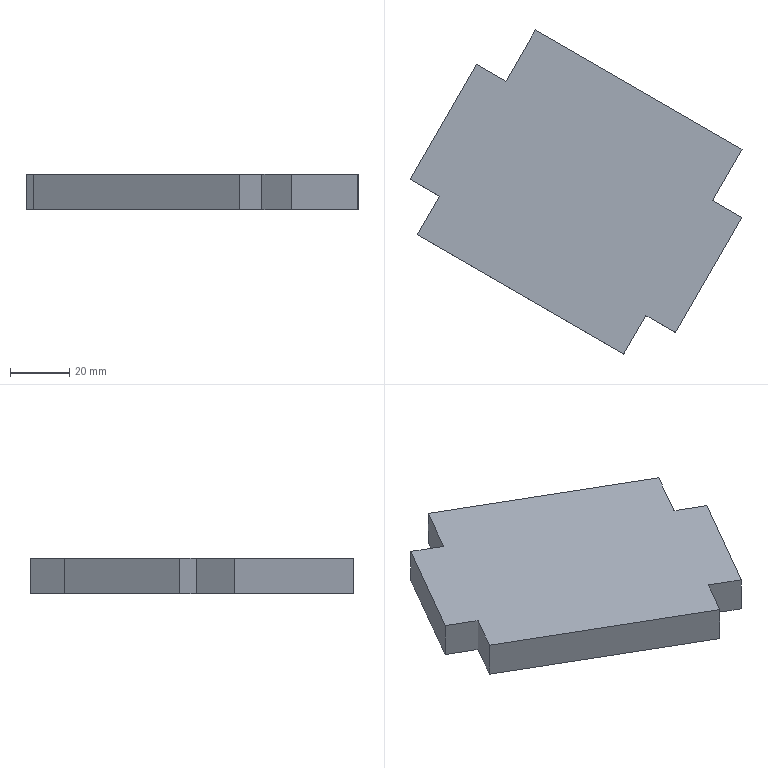Part | SolidWorks | features FlatPattern 1, SMBaseFlange 1, SheetMetal 1 | 1 solid | 14 faces | box 112.348 x 109.632 x 12 mm | volume 89892 mm3 | plane 14
STEP:
#1=CARTESIAN_POINT('',(-12.686,188.938,0.));
#2=VERTEX_POINT('',#1);
#3=CARTESIAN_POINT('',(-22.686,171.617,0.));
#4=VERTEX_POINT('',#3);
#5=CARTESIAN_POINT('',(-22.686,171.617,0.));
#6=DIRECTION('',(-0.5,-0.866,0.));
#7=VECTOR('',#6,1000.);
#8=LINE('',#5,#7);
#9=EDGE_CURVE('',#2,#4,#8,.T.);
#10=ORIENTED_EDGE('',*,*,#9,.F.);
#11=CARTESIAN_POINT('',(-12.686,188.938,-12.));
#12=VERTEX_POINT('',#11);
#13=CARTESIAN_POINT('',(-12.686,188.938,-12.));
#14=DIRECTION('',(0.,0.,1.));
#15=VECTOR('',#14,1000.);
#16=LINE('',#13,#15);
#17=EDGE_CURVE('',#12,#2,#16,.T.);
#18=ORIENTED_EDGE('',*,*,#17,.F.);
#19=CARTESIAN_POINT('',(-22.686,171.617,-12.));
#20=VERTEX_POINT('',#19);
#21=CARTESIAN_POINT('',(-22.686,171.617,-12.));
#22=DIRECTION('',(-0.5,-0.866,0.));
#23=VECTOR('',#22,1000.);
#24=LINE('',#21,#23);
#25=EDGE_CURVE('',#12,#20,#24,.T.);
#26=ORIENTED_EDGE('',*,*,#25,.T.);
#27=CARTESIAN_POINT('',(-22.686,171.617,-12.));
#28=DIRECTION('',(0.,0.,1.));
#29=VECTOR('',#28,1000.);
#30=LINE('',#27,#29);
#31=EDGE_CURVE('',#20,#4,#30,.T.);
#32=ORIENTED_EDGE('',*,*,#31,.T.);
#33=EDGE_LOOP('',(#10,#18,#26,#32));
#34=FACE_OUTER_BOUND('',#33,.T.);
#35=CARTESIAN_POINT('',(-22.686,171.617,-12.));
#36=DIRECTION('',(-0.866,0.5,0.));
#37=DIRECTION('',(-0.5,-0.866,0.));
#38=AXIS2_PLACEMENT_3D('',#35,#36,#37);
#39=PLANE('',#38);
#40=ADVANCED_FACE('',(#34),#39,.T.);
#41=CARTESIAN_POINT('',(57.203,148.588,0.));
#42=VERTEX_POINT('',#41);
#43=CARTESIAN_POINT('',(-12.686,188.938,0.));
#44=DIRECTION('',(-0.866,0.5,0.));
#45=VECTOR('',#44,1000.);
#46=LINE('',#43,#45);
#47=EDGE_CURVE('',#42,#2,#46,.T.);
#48=ORIENTED_EDGE('',*,*,#47,.F.);
#49=CARTESIAN_POINT('',(57.203,148.588,-12.));
#50=VERTEX_POINT('',#49);
#51=CARTESIAN_POINT('',(57.203,148.588,-12.));
#52=DIRECTION('',(0.,0.,1.));
#53=VECTOR('',#52,1000.);
#54=LINE('',#51,#53);
#55=EDGE_CURVE('',#50,#42,#54,.T.);
#56=ORIENTED_EDGE('',*,*,#55,.F.);
#57=CARTESIAN_POINT('',(-12.686,188.938,-12.));
#58=DIRECTION('',(-0.866,0.5,0.));
#59=VECTOR('',#58,1000.);
#60=LINE('',#57,#59);
#61=EDGE_CURVE('',#50,#12,#60,.T.);
#62=ORIENTED_EDGE('',*,*,#61,.T.);
#63=ORIENTED_EDGE('',*,*,#17,.T.);
#64=EDGE_LOOP('',(#48,#56,#62,#63));
#65=FACE_OUTER_BOUND('',#64,.T.);
#66=CARTESIAN_POINT('',(-12.686,188.938,-12.));
#67=DIRECTION('',(0.5,0.866,0.));
#68=DIRECTION('',(-0.866,0.5,0.));
#69=AXIS2_PLACEMENT_3D('',#66,#67,#68);
#70=PLANE('',#69);
#71=ADVANCED_FACE('',(#65),#70,.T.);
#72=CARTESIAN_POINT('',(47.203,131.267,0.));
#73=VERTEX_POINT('',#72);
#74=CARTESIAN_POINT('',(57.203,148.588,0.));
#75=DIRECTION('',(0.5,0.866,0.));
#76=VECTOR('',#75,1000.);
#77=LINE('',#74,#76);
#78=EDGE_CURVE('',#73,#42,#77,.T.);
#79=ORIENTED_EDGE('',*,*,#78,.F.);
#80=CARTESIAN_POINT('',(47.203,131.267,-12.));
#81=VERTEX_POINT('',#80);
#82=CARTESIAN_POINT('',(47.203,131.267,-12.));
#83=DIRECTION('',(0.,0.,1.));
#84=VECTOR('',#83,1000.);
#85=LINE('',#82,#84);
#86=EDGE_CURVE('',#81,#73,#85,.T.);
#87=ORIENTED_EDGE('',*,*,#86,.F.);
#88=CARTESIAN_POINT('',(57.203,148.588,-12.));
#89=DIRECTION('',(0.5,0.866,0.));
#90=VECTOR('',#89,1000.);
#91=LINE('',#88,#90);
#92=EDGE_CURVE('',#81,#50,#91,.T.);
#93=ORIENTED_EDGE('',*,*,#92,.T.);
#94=ORIENTED_EDGE('',*,*,#55,.T.);
#95=EDGE_LOOP('',(#79,#87,#93,#94));
#96=FACE_OUTER_BOUND('',#95,.T.);
#97=CARTESIAN_POINT('',(57.203,148.588,-12.));
#98=DIRECTION('',(0.866,-0.5,0.));
#99=DIRECTION('',(0.5,0.866,0.));
#100=AXIS2_PLACEMENT_3D('',#97,#98,#99);
#101=PLANE('',#100);
#102=ADVANCED_FACE('',(#96),#101,.T.);
#103=CARTESIAN_POINT('',(57.162,125.517,0.));
#104=VERTEX_POINT('',#103);
#105=CARTESIAN_POINT('',(57.162,125.517,0.));
#106=DIRECTION('',(-0.866,0.5,0.));
#107=VECTOR('',#106,1000.);
#108=LINE('',#105,#107);
#109=EDGE_CURVE('',#104,#73,#108,.T.);
#110=ORIENTED_EDGE('',*,*,#109,.F.);
#111=CARTESIAN_POINT('',(57.162,125.517,-12.));
#112=VERTEX_POINT('',#111);
#113=CARTESIAN_POINT('',(57.162,125.517,-12.));
#114=DIRECTION('',(0.,0.,1.));
#115=VECTOR('',#114,1000.);
#116=LINE('',#113,#115);
#117=EDGE_CURVE('',#112,#104,#116,.T.);
#118=ORIENTED_EDGE('',*,*,#117,.F.);
#119=CARTESIAN_POINT('',(57.162,125.517,-12.));
#120=DIRECTION('',(-0.866,0.5,0.));
#121=VECTOR('',#120,1000.);
#122=LINE('',#119,#121);
#123=EDGE_CURVE('',#112,#81,#122,.T.);
#124=ORIENTED_EDGE('',*,*,#123,.T.);
#125=ORIENTED_EDGE('',*,*,#86,.T.);
#126=EDGE_LOOP('',(#110,#118,#124,#125));
#127=FACE_OUTER_BOUND('',#126,.T.);
#128=CARTESIAN_POINT('',(57.162,125.517,-12.));
#129=DIRECTION('',(0.5,0.866,0.));
#130=DIRECTION('',(-0.866,0.5,0.));
#131=AXIS2_PLACEMENT_3D('',#128,#129,#130);
#132=PLANE('',#131);
#133=ADVANCED_FACE('',(#127),#132,.T.);
#134=CARTESIAN_POINT('',(34.662,86.546,0.));
#135=VERTEX_POINT('',#134);
#136=CARTESIAN_POINT('',(34.662,86.546,0.));
#137=DIRECTION('',(0.5,0.866,0.));
#138=VECTOR('',#137,1000.);
#139=LINE('',#136,#138);
#140=EDGE_CURVE('',#135,#104,#139,.T.);
#141=ORIENTED_EDGE('',*,*,#140,.F.);
#142=CARTESIAN_POINT('',(34.662,86.546,-12.));
#143=VERTEX_POINT('',#142);
#144=CARTESIAN_POINT('',(34.662,86.546,-12.));
#145=DIRECTION('',(0.,0.,1.));
#146=VECTOR('',#145,1000.);
#147=LINE('',#144,#146);
#148=EDGE_CURVE('',#143,#135,#147,.T.);
#149=ORIENTED_EDGE('',*,*,#148,.F.);
#150=CARTESIAN_POINT('',(34.662,86.546,-12.));
#151=DIRECTION('',(0.5,0.866,0.));
#152=VECTOR('',#151,1000.);
#153=LINE('',#150,#152);
#154=EDGE_CURVE('',#143,#112,#153,.T.);
#155=ORIENTED_EDGE('',*,*,#154,.T.);
#156=ORIENTED_EDGE('',*,*,#117,.T.);
#157=EDGE_LOOP('',(#141,#149,#155,#156));
#158=FACE_OUTER_BOUND('',#157,.T.);
#159=CARTESIAN_POINT('',(34.662,86.546,-12.));
#160=DIRECTION('',(0.866,-0.5,0.));
#161=DIRECTION('',(0.5,0.866,0.));
#162=AXIS2_PLACEMENT_3D('',#159,#160,#161);
#163=PLANE('',#162);
#164=ADVANCED_FACE('',(#158),#163,.T.);
#165=CARTESIAN_POINT('',(24.703,92.296,0.));
#166=VERTEX_POINT('',#165);
#167=CARTESIAN_POINT('',(24.703,92.296,0.));
#168=DIRECTION('',(0.866,-0.5,0.));
#169=VECTOR('',#168,1000.);
#170=LINE('',#167,#169);
#171=EDGE_CURVE('',#166,#135,#170,.T.);
#172=ORIENTED_EDGE('',*,*,#171,.F.);
#173=CARTESIAN_POINT('',(24.703,92.296,-12.));
#174=VERTEX_POINT('',#173);
#175=CARTESIAN_POINT('',(24.703,92.296,-12.));
#176=DIRECTION('',(0.,0.,1.));
#177=VECTOR('',#176,1000.);
#178=LINE('',#175,#177);
#179=EDGE_CURVE('',#174,#166,#178,.T.);
#180=ORIENTED_EDGE('',*,*,#179,.F.);
#181=CARTESIAN_POINT('',(24.703,92.296,-12.));
#182=DIRECTION('',(0.866,-0.5,0.));
#183=VECTOR('',#182,1000.);
#184=LINE('',#181,#183);
#185=EDGE_CURVE('',#174,#143,#184,.T.);
#186=ORIENTED_EDGE('',*,*,#185,.T.);
#187=ORIENTED_EDGE('',*,*,#148,.T.);
#188=EDGE_LOOP('',(#172,#180,#186,#187));
#189=FACE_OUTER_BOUND('',#188,.T.);
#190=CARTESIAN_POINT('',(24.703,92.296,-12.));
#191=DIRECTION('',(-0.5,-0.866,0.));
#192=DIRECTION('',(0.866,-0.5,0.));
#193=AXIS2_PLACEMENT_3D('',#190,#191,#192);
#194=PLANE('',#193);
#195=ADVANCED_FACE('',(#189),#194,.T.);
#196=CARTESIAN_POINT('',(17.203,79.306,0.));
#197=VERTEX_POINT('',#196);
#198=CARTESIAN_POINT('',(24.703,92.296,0.));
#199=DIRECTION('',(0.5,0.866,0.));
#200=VECTOR('',#199,1000.);
#201=LINE('',#198,#200);
#202=EDGE_CURVE('',#197,#166,#201,.T.);
#203=ORIENTED_EDGE('',*,*,#202,.F.);
#204=CARTESIAN_POINT('',(17.203,79.306,-12.));
#205=VERTEX_POINT('',#204);
#206=CARTESIAN_POINT('',(17.203,79.306,-12.));
#207=DIRECTION('',(0.,0.,1.));
#208=VECTOR('',#207,1000.);
#209=LINE('',#206,#208);
#210=EDGE_CURVE('',#205,#197,#209,.T.);
#211=ORIENTED_EDGE('',*,*,#210,.F.);
#212=CARTESIAN_POINT('',(24.703,92.296,-12.));
#213=DIRECTION('',(0.5,0.866,0.));
#214=VECTOR('',#213,1000.);
#215=LINE('',#212,#214);
#216=EDGE_CURVE('',#205,#174,#215,.T.);
#217=ORIENTED_EDGE('',*,*,#216,.T.);
#218=ORIENTED_EDGE('',*,*,#179,.T.);
#219=EDGE_LOOP('',(#203,#211,#217,#218));
#220=FACE_OUTER_BOUND('',#219,.T.);
#221=CARTESIAN_POINT('',(24.703,92.296,-12.));
#222=DIRECTION('',(0.866,-0.5,0.));
#223=DIRECTION('',(0.5,0.866,0.));
#224=AXIS2_PLACEMENT_3D('',#221,#222,#223);
#225=PLANE('',#224);
#226=ADVANCED_FACE('',(#220),#225,.T.);
#227=CARTESIAN_POINT('',(-52.686,119.656,0.));
#228=VERTEX_POINT('',#227);
#229=CARTESIAN_POINT('',(17.203,79.306,0.));
#230=DIRECTION('',(0.866,-0.5,0.));
#231=VECTOR('',#230,1000.);
#232=LINE('',#229,#231);
#233=EDGE_CURVE('',#228,#197,#232,.T.);
#234=ORIENTED_EDGE('',*,*,#233,.F.);
#235=CARTESIAN_POINT('',(-52.686,119.656,-12.));
#236=VERTEX_POINT('',#235);
#237=CARTESIAN_POINT('',(-52.686,119.656,-12.));
#238=DIRECTION('',(0.,0.,1.));
#239=VECTOR('',#238,1000.);
#240=LINE('',#237,#239);
#241=EDGE_CURVE('',#236,#228,#240,.T.);
#242=ORIENTED_EDGE('',*,*,#241,.F.);
#243=CARTESIAN_POINT('',(17.203,79.306,-12.));
#244=DIRECTION('',(0.866,-0.5,0.));
#245=VECTOR('',#244,1000.);
#246=LINE('',#243,#245);
#247=EDGE_CURVE('',#236,#205,#246,.T.);
#248=ORIENTED_EDGE('',*,*,#247,.T.);
#249=ORIENTED_EDGE('',*,*,#210,.T.);
#250=EDGE_LOOP('',(#234,#242,#248,#249));
#251=FACE_OUTER_BOUND('',#250,.T.);
#252=CARTESIAN_POINT('',(17.203,79.306,-12.));
#253=DIRECTION('',(-0.5,-0.866,0.));
#254=DIRECTION('',(0.866,-0.5,0.));
#255=AXIS2_PLACEMENT_3D('',#252,#253,#254);
#256=PLANE('',#255);
#257=ADVANCED_FACE('',(#251),#256,.T.);
#258=CARTESIAN_POINT('',(-45.186,132.646,0.));
#259=VERTEX_POINT('',#258);
#260=CARTESIAN_POINT('',(-52.686,119.656,0.));
#261=DIRECTION('',(-0.5,-0.866,0.));
#262=VECTOR('',#261,1000.);
#263=LINE('',#260,#262);
#264=EDGE_CURVE('',#259,#228,#263,.T.);
#265=ORIENTED_EDGE('',*,*,#264,.F.);
#266=CARTESIAN_POINT('',(-45.186,132.646,-12.));
#267=VERTEX_POINT('',#266);
#268=CARTESIAN_POINT('',(-45.186,132.646,-12.));
#269=DIRECTION('',(0.,0.,1.));
#270=VECTOR('',#269,1000.);
#271=LINE('',#268,#270);
#272=EDGE_CURVE('',#267,#259,#271,.T.);
#273=ORIENTED_EDGE('',*,*,#272,.F.);
#274=CARTESIAN_POINT('',(-52.686,119.656,-12.));
#275=DIRECTION('',(-0.5,-0.866,0.));
#276=VECTOR('',#275,1000.);
#277=LINE('',#274,#276);
#278=EDGE_CURVE('',#267,#236,#277,.T.);
#279=ORIENTED_EDGE('',*,*,#278,.T.);
#280=ORIENTED_EDGE('',*,*,#241,.T.);
#281=EDGE_LOOP('',(#265,#273,#279,#280));
#282=FACE_OUTER_BOUND('',#281,.T.);
#283=CARTESIAN_POINT('',(-52.686,119.656,-12.));
#284=DIRECTION('',(-0.866,0.5,0.));
#285=DIRECTION('',(-0.5,-0.866,0.));
#286=AXIS2_PLACEMENT_3D('',#283,#284,#285);
#287=PLANE('',#286);
#288=ADVANCED_FACE('',(#282),#287,.T.);
#289=CARTESIAN_POINT('',(-55.145,138.396,0.));
#290=VERTEX_POINT('',#289);
#291=CARTESIAN_POINT('',(-45.186,132.646,0.));
#292=DIRECTION('',(0.866,-0.5,0.));
#293=VECTOR('',#292,1000.);
#294=LINE('',#291,#293);
#295=EDGE_CURVE('',#290,#259,#294,.T.);
#296=ORIENTED_EDGE('',*,*,#295,.F.);
#297=CARTESIAN_POINT('',(-55.145,138.396,-12.));
#298=VERTEX_POINT('',#297);
#299=CARTESIAN_POINT('',(-55.145,138.396,-12.));
#300=DIRECTION('',(0.,0.,1.));
#301=VECTOR('',#300,1000.);
#302=LINE('',#299,#301);
#303=EDGE_CURVE('',#298,#290,#302,.T.);
#304=ORIENTED_EDGE('',*,*,#303,.F.);
#305=CARTESIAN_POINT('',(-45.186,132.646,-12.));
#306=DIRECTION('',(0.866,-0.5,0.));
#307=VECTOR('',#306,1000.);
#308=LINE('',#305,#307);
#309=EDGE_CURVE('',#298,#267,#308,.T.);
#310=ORIENTED_EDGE('',*,*,#309,.T.);
#311=ORIENTED_EDGE('',*,*,#272,.T.);
#312=EDGE_LOOP('',(#296,#304,#310,#311));
#313=FACE_OUTER_BOUND('',#312,.T.);
#314=CARTESIAN_POINT('',(-45.186,132.646,-12.));
#315=DIRECTION('',(-0.5,-0.866,0.));
#316=DIRECTION('',(0.866,-0.5,0.));
#317=AXIS2_PLACEMENT_3D('',#314,#315,#316);
#318=PLANE('',#317);
#319=ADVANCED_FACE('',(#313),#318,.T.);
#320=CARTESIAN_POINT('',(-32.645,177.367,0.));
#321=VERTEX_POINT('',#320);
#322=CARTESIAN_POINT('',(-55.145,138.396,0.));
#323=DIRECTION('',(-0.5,-0.866,0.));
#324=VECTOR('',#323,1000.);
#325=LINE('',#322,#324);
#326=EDGE_CURVE('',#321,#290,#325,.T.);
#327=ORIENTED_EDGE('',*,*,#326,.F.);
#328=CARTESIAN_POINT('',(-32.645,177.367,-12.));
#329=VERTEX_POINT('',#328);
#330=CARTESIAN_POINT('',(-32.645,177.367,-12.));
#331=DIRECTION('',(0.,0.,1.));
#332=VECTOR('',#331,1000.);
#333=LINE('',#330,#332);
#334=EDGE_CURVE('',#329,#321,#333,.T.);
#335=ORIENTED_EDGE('',*,*,#334,.F.);
#336=CARTESIAN_POINT('',(-55.145,138.396,-12.));
#337=DIRECTION('',(-0.5,-0.866,0.));
#338=VECTOR('',#337,1000.);
#339=LINE('',#336,#338);
#340=EDGE_CURVE('',#329,#298,#339,.T.);
#341=ORIENTED_EDGE('',*,*,#340,.T.);
#342=ORIENTED_EDGE('',*,*,#303,.T.);
#343=EDGE_LOOP('',(#327,#335,#341,#342));
#344=FACE_OUTER_BOUND('',#343,.T.);
#345=CARTESIAN_POINT('',(-55.145,138.396,-12.));
#346=DIRECTION('',(-0.866,0.5,0.));
#347=DIRECTION('',(-0.5,-0.866,0.));
#348=AXIS2_PLACEMENT_3D('',#345,#346,#347);
#349=PLANE('',#348);
#350=ADVANCED_FACE('',(#344),#349,.T.);
#351=CARTESIAN_POINT('',(-32.645,177.367,0.));
#352=DIRECTION('',(-0.866,0.5,0.));
#353=VECTOR('',#352,1000.);
#354=LINE('',#351,#353);
#355=EDGE_CURVE('',#4,#321,#354,.T.);
#356=ORIENTED_EDGE('',*,*,#355,.F.);
#357=ORIENTED_EDGE('',*,*,#31,.F.);
#358=CARTESIAN_POINT('',(-32.645,177.367,-12.));
#359=DIRECTION('',(-0.866,0.5,0.));
#360=VECTOR('',#359,1000.);
#361=LINE('',#358,#360);
#362=EDGE_CURVE('',#20,#329,#361,.T.);
#363=ORIENTED_EDGE('',*,*,#362,.T.);
#364=ORIENTED_EDGE('',*,*,#334,.T.);
#365=EDGE_LOOP('',(#356,#357,#363,#364));
#366=FACE_OUTER_BOUND('',#365,.T.);
#367=CARTESIAN_POINT('',(-32.645,177.367,-12.));
#368=DIRECTION('',(0.5,0.866,0.));
#369=DIRECTION('',(-0.866,0.5,0.));
#370=AXIS2_PLACEMENT_3D('',#367,#368,#369);
#371=PLANE('',#370);
#372=ADVANCED_FACE('',(#366),#371,.T.);
#373=ORIENTED_EDGE('',*,*,#25,.F.);
#374=ORIENTED_EDGE('',*,*,#61,.F.);
#375=ORIENTED_EDGE('',*,*,#92,.F.);
#376=ORIENTED_EDGE('',*,*,#123,.F.);
#377=ORIENTED_EDGE('',*,*,#154,.F.);
#378=ORIENTED_EDGE('',*,*,#185,.F.);
#379=ORIENTED_EDGE('',*,*,#216,.F.);
#380=ORIENTED_EDGE('',*,*,#247,.F.);
#381=ORIENTED_EDGE('',*,*,#278,.F.);
#382=ORIENTED_EDGE('',*,*,#309,.F.);
#383=ORIENTED_EDGE('',*,*,#340,.F.);
#384=ORIENTED_EDGE('',*,*,#362,.F.);
#385=EDGE_LOOP('',(#373,#374,#375,#376,#377,#378,#379,#380,#381,#382,#383,#384));
#386=FACE_OUTER_BOUND('',#385,.T.);
#387=CARTESIAN_POINT('',(0.,0.,-12.));
#388=DIRECTION('',(0.,0.,-1.));
#389=DIRECTION('',(-1.,0.,0.));
#390=AXIS2_PLACEMENT_3D('',#387,#388,#389);
#391=PLANE('',#390);
#392=ADVANCED_FACE('',(#386),#391,.T.);
#393=ORIENTED_EDGE('',*,*,#9,.T.);
#394=ORIENTED_EDGE('',*,*,#355,.T.);
#395=ORIENTED_EDGE('',*,*,#326,.T.);
#396=ORIENTED_EDGE('',*,*,#295,.T.);
#397=ORIENTED_EDGE('',*,*,#264,.T.);
#398=ORIENTED_EDGE('',*,*,#233,.T.);
#399=ORIENTED_EDGE('',*,*,#202,.T.);
#400=ORIENTED_EDGE('',*,*,#171,.T.);
#401=ORIENTED_EDGE('',*,*,#140,.T.);
#402=ORIENTED_EDGE('',*,*,#109,.T.);
#403=ORIENTED_EDGE('',*,*,#78,.T.);
#404=ORIENTED_EDGE('',*,*,#47,.T.);
#405=EDGE_LOOP('',(#393,#394,#395,#396,#397,#398,#399,#400,#401,#402,#403,#404));
#406=FACE_OUTER_BOUND('',#405,.T.);
#407=CARTESIAN_POINT('',(0.,0.,0.));
#408=DIRECTION('',(0.,0.,-1.));
#409=DIRECTION('',(-1.,0.,0.));
#410=AXIS2_PLACEMENT_3D('',#407,#408,#409);
#411=PLANE('',#410);
#412=ADVANCED_FACE('',(#406),#411,.F.);
#413=CLOSED_SHELL('',(#40,#71,#102,#133,#164,#195,#226,#257,#288,#319,#350,#372,#392,#412));
#414=MANIFOLD_SOLID_BREP('',#413);
#415=CARTESIAN_POINT('',(0.,0.,0.));
#416=DIRECTION('',(0.,0.,1.));
#417=DIRECTION('',(1.,0.,0.));
#418=AXIS2_PLACEMENT_3D('',#415,#416,#417);
#419=(LENGTH_UNIT()NAMED_UNIT(*)SI_UNIT(.MILLI.,.METRE.));
#420=UNCERTAINTY_MEASURE_WITH_UNIT(LENGTH_MEASURE(0.00001),#419,'','');
#421=(NAMED_UNIT(*)PLANE_ANGLE_UNIT()SI_UNIT($,.RADIAN.));
#422=(NAMED_UNIT(*)SI_UNIT($,.STERADIAN.)SOLID_ANGLE_UNIT());
#423=(GEOMETRIC_REPRESENTATION_CONTEXT(3)GLOBAL_UNCERTAINTY_ASSIGNED_CONTEXT((#420))GLOBAL_UNIT_ASSIGNED_CONTEXT((#419,#421,#422))REPRESENTATION_CONTEXT('',''));
#424=ADVANCED_BREP_SHAPE_REPRESENTATION('',(#414,#418),#423);